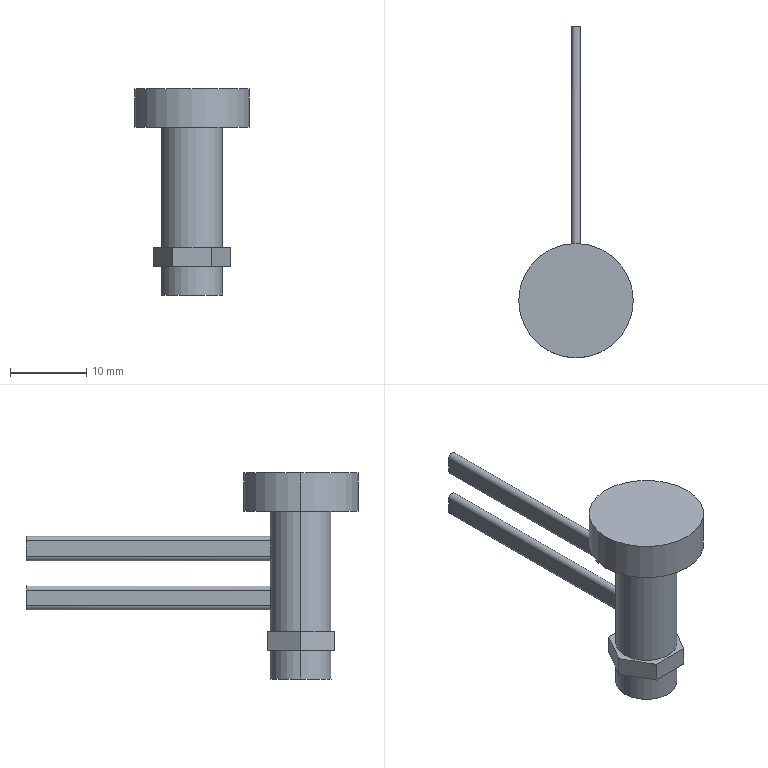Part | SolidWorks | features BaseBody 1 | 1 solid | 29 faces | box 15 x 43.5 x 27 mm | volume 2257 mm3 | plane 17 | cylinder 12 | commonest cylinder face diameters 1.197 x6 8 x4 15 x2
STEP:
#1=CARTESIAN_POINT('',(0.,36.,-12.942));
#2=VERTEX_POINT('',#1);
#3=CARTESIAN_POINT('',(-0.5985,36.,-12.344));
#4=VERTEX_POINT('',#3);
#5=CARTESIAN_POINT('',(0.,36.,-12.344));
#6=DIRECTION('',(0.,1.,0.));
#7=DIRECTION('',(0.,0.,1.));
#8=AXIS2_PLACEMENT_3D('',#5,#6,#7);
#9=CIRCLE('',#8,0.5985);
#10=EDGE_CURVE('',#2,#4,#9,.T.);
#11=ORIENTED_EDGE('',*,*,#10,.F.);
#12=CARTESIAN_POINT('',(0.,4.,-12.942));
#13=VERTEX_POINT('',#12);
#14=CARTESIAN_POINT('',(0.,36.,-12.942));
#15=DIRECTION('',(0.,-1.,0.));
#16=VECTOR('',#15,1000.);
#17=LINE('',#14,#16);
#18=EDGE_CURVE('',#2,#13,#17,.T.);
#19=ORIENTED_EDGE('',*,*,#18,.T.);
#20=CARTESIAN_POINT('',(-0.5985,3.955,-12.344));
#21=VERTEX_POINT('',#20);
#22=CARTESIAN_POINT('',(0.,4.,-12.942));
#23=CARTESIAN_POINT('',(-0.1585,4.,-12.942));
#24=CARTESIAN_POINT('',(-0.3131,3.989,-12.877));
#25=CARTESIAN_POINT('',(-0.5336,3.966,-12.657));
#26=CARTESIAN_POINT('',(-0.5985,3.955,-12.5));
#27=CARTESIAN_POINT('',(-0.5985,3.955,-12.344));
#28=B_SPLINE_CURVE_WITH_KNOTS('',3,(#22,#23,#24,#25,#26,#27),.UNSPECIFIED.,.F.,.F.,(4,2,4),(0.,0.0004686,0.0009371),.UNSPECIFIED.);
#29=EDGE_CURVE('',#13,#21,#28,.T.);
#30=ORIENTED_EDGE('',*,*,#29,.T.);
#31=CARTESIAN_POINT('',(-0.5985,36.,-12.344));
#32=DIRECTION('',(0.,-1.,0.));
#33=VECTOR('',#32,1000.);
#34=LINE('',#31,#33);
#35=EDGE_CURVE('',#4,#21,#34,.T.);
#36=ORIENTED_EDGE('',*,*,#35,.F.);
#37=EDGE_LOOP('',(#11,#19,#30,#36));
#38=FACE_OUTER_BOUND('',#37,.T.);
#39=CARTESIAN_POINT('',(0.,36.,-12.344));
#40=DIRECTION('',(0.,-1.,0.));
#41=DIRECTION('',(0.,0.,-1.));
#42=AXIS2_PLACEMENT_3D('',#39,#40,#41);
#43=CYLINDRICAL_SURFACE('',#42,0.5985);
#44=ADVANCED_FACE('',(#38),#43,.T.);
#45=CARTESIAN_POINT('',(0.,36.,-6.501));
#46=VERTEX_POINT('',#45);
#47=CARTESIAN_POINT('',(-0.5985,36.,-5.903));
#48=VERTEX_POINT('',#47);
#49=CARTESIAN_POINT('',(0.,36.,-5.903));
#50=DIRECTION('',(0.,1.,0.));
#51=DIRECTION('',(0.,0.,1.));
#52=AXIS2_PLACEMENT_3D('',#49,#50,#51);
#53=CIRCLE('',#52,0.5985);
#54=EDGE_CURVE('',#46,#48,#53,.T.);
#55=ORIENTED_EDGE('',*,*,#54,.F.);
#56=CARTESIAN_POINT('',(0.,4.,-6.501));
#57=VERTEX_POINT('',#56);
#58=CARTESIAN_POINT('',(0.,36.,-6.501));
#59=DIRECTION('',(0.,-1.,0.));
#60=VECTOR('',#59,1000.);
#61=LINE('',#58,#60);
#62=EDGE_CURVE('',#46,#57,#61,.T.);
#63=ORIENTED_EDGE('',*,*,#62,.T.);
#64=CARTESIAN_POINT('',(-0.5985,3.955,-5.903));
#65=VERTEX_POINT('',#64);
#66=CARTESIAN_POINT('',(0.,4.,-6.501));
#67=CARTESIAN_POINT('',(-0.1585,4.,-6.501));
#68=CARTESIAN_POINT('',(-0.3131,3.989,-6.436));
#69=CARTESIAN_POINT('',(-0.5336,3.966,-6.216));
#70=CARTESIAN_POINT('',(-0.5985,3.955,-6.059));
#71=CARTESIAN_POINT('',(-0.5985,3.955,-5.903));
#72=B_SPLINE_CURVE_WITH_KNOTS('',3,(#66,#67,#68,#69,#70,#71),.UNSPECIFIED.,.F.,.F.,(4,2,4),(0.,0.0004686,0.0009371),.UNSPECIFIED.);
#73=EDGE_CURVE('',#57,#65,#72,.T.);
#74=ORIENTED_EDGE('',*,*,#73,.T.);
#75=CARTESIAN_POINT('',(-0.5985,36.,-5.903));
#76=DIRECTION('',(0.,-1.,0.));
#77=VECTOR('',#76,1000.);
#78=LINE('',#75,#77);
#79=EDGE_CURVE('',#48,#65,#78,.T.);
#80=ORIENTED_EDGE('',*,*,#79,.F.);
#81=EDGE_LOOP('',(#55,#63,#74,#80));
#82=FACE_OUTER_BOUND('',#81,.T.);
#83=CARTESIAN_POINT('',(0.,36.,-5.903));
#84=DIRECTION('',(0.,-1.,0.));
#85=DIRECTION('',(0.,0.,-1.));
#86=AXIS2_PLACEMENT_3D('',#83,#84,#85);
#87=CYLINDRICAL_SURFACE('',#86,0.5985);
#88=ADVANCED_FACE('',(#82),#87,.T.);
#89=CARTESIAN_POINT('',(-4.,0.,-22.));
#90=VERTEX_POINT('',#89);
#91=CARTESIAN_POINT('',(4.,0.,-22.));
#92=VERTEX_POINT('',#91);
#93=CARTESIAN_POINT('',(0.,0.,-22.));
#94=DIRECTION('',(0.,0.,-1.));
#95=DIRECTION('',(-1.,0.,0.));
#96=AXIS2_PLACEMENT_3D('',#93,#94,#95);
#97=CIRCLE('',#96,4.);
#98=EDGE_CURVE('',#90,#92,#97,.T.);
#99=ORIENTED_EDGE('',*,*,#98,.F.);
#100=CARTESIAN_POINT('',(-4.,0.,-18.25));
#101=VERTEX_POINT('',#100);
#102=CARTESIAN_POINT('',(-4.,0.,-22.));
#103=DIRECTION('',(0.,0.,1.));
#104=VECTOR('',#103,1000.);
#105=LINE('',#102,#104);
#106=EDGE_CURVE('',#90,#101,#105,.T.);
#107=ORIENTED_EDGE('',*,*,#106,.T.);
#108=CARTESIAN_POINT('',(4.,0.,-18.25));
#109=VERTEX_POINT('',#108);
#110=CARTESIAN_POINT('',(0.,0.,-18.25));
#111=DIRECTION('',(0.,0.,-1.));
#112=DIRECTION('',(-1.,0.,0.));
#113=AXIS2_PLACEMENT_3D('',#110,#111,#112);
#114=CIRCLE('',#113,4.);
#115=EDGE_CURVE('',#101,#109,#114,.T.);
#116=ORIENTED_EDGE('',*,*,#115,.T.);
#117=CARTESIAN_POINT('',(4.,0.,-22.));
#118=DIRECTION('',(0.,0.,1.));
#119=VECTOR('',#118,1000.);
#120=LINE('',#117,#119);
#121=EDGE_CURVE('',#92,#109,#120,.T.);
#122=ORIENTED_EDGE('',*,*,#121,.F.);
#123=EDGE_LOOP('',(#99,#107,#116,#122));
#124=FACE_OUTER_BOUND('',#123,.T.);
#125=CARTESIAN_POINT('',(0.,0.,-22.));
#126=DIRECTION('',(0.,0.,1.));
#127=DIRECTION('',(1.,0.,0.));
#128=AXIS2_PLACEMENT_3D('',#125,#126,#127);
#129=CYLINDRICAL_SURFACE('',#128,4.);
#130=ADVANCED_FACE('',(#124),#129,.T.);
#131=CARTESIAN_POINT('',(7.5,0.,5.));
#132=VERTEX_POINT('',#131);
#133=CARTESIAN_POINT('',(-7.5,0.,5.));
#134=VERTEX_POINT('',#133);
#135=CARTESIAN_POINT('',(0.,0.,5.));
#136=DIRECTION('',(0.,0.,1.));
#137=DIRECTION('',(1.,0.,0.));
#138=AXIS2_PLACEMENT_3D('',#135,#136,#137);
#139=CIRCLE('',#138,7.5);
#140=EDGE_CURVE('',#132,#134,#139,.T.);
#141=ORIENTED_EDGE('',*,*,#140,.F.);
#142=CARTESIAN_POINT('',(7.5,0.,0.));
#143=VERTEX_POINT('',#142);
#144=CARTESIAN_POINT('',(7.5,0.,5.));
#145=DIRECTION('',(0.,0.,-1.));
#146=VECTOR('',#145,1000.);
#147=LINE('',#144,#146);
#148=EDGE_CURVE('',#132,#143,#147,.T.);
#149=ORIENTED_EDGE('',*,*,#148,.T.);
#150=CARTESIAN_POINT('',(-7.5,0.,0.));
#151=VERTEX_POINT('',#150);
#152=CARTESIAN_POINT('',(0.,0.,0.));
#153=DIRECTION('',(0.,0.,1.));
#154=DIRECTION('',(1.,0.,0.));
#155=AXIS2_PLACEMENT_3D('',#152,#153,#154);
#156=CIRCLE('',#155,7.5);
#157=EDGE_CURVE('',#143,#151,#156,.T.);
#158=ORIENTED_EDGE('',*,*,#157,.T.);
#159=CARTESIAN_POINT('',(-7.5,0.,5.));
#160=DIRECTION('',(0.,0.,-1.));
#161=VECTOR('',#160,1000.);
#162=LINE('',#159,#161);
#163=EDGE_CURVE('',#134,#151,#162,.T.);
#164=ORIENTED_EDGE('',*,*,#163,.F.);
#165=EDGE_LOOP('',(#141,#149,#158,#164));
#166=FACE_OUTER_BOUND('',#165,.T.);
#167=CARTESIAN_POINT('',(0.,0.,5.));
#168=DIRECTION('',(0.,0.,-1.));
#169=DIRECTION('',(-1.,0.,0.));
#170=AXIS2_PLACEMENT_3D('',#167,#168,#169);
#171=CYLINDRICAL_SURFACE('',#170,7.5);
#172=ADVANCED_FACE('',(#166),#171,.T.);
#173=CARTESIAN_POINT('',(-0.5985,3.955,-3.903));
#174=VERTEX_POINT('',#173);
#175=CARTESIAN_POINT('',(0.5985,3.955,-3.903));
#176=VERTEX_POINT('',#175);
#177=CARTESIAN_POINT('',(-0.5985,3.955,-3.903));
#178=CARTESIAN_POINT('',(-0.5985,3.955,-3.746));
#179=CARTESIAN_POINT('',(-0.5347,3.966,-3.591));
#180=CARTESIAN_POINT('',(-0.3115,3.989,-3.368));
#181=CARTESIAN_POINT('',(-0.1562,4.,-3.304));
#182=CARTESIAN_POINT('',(0.1565,4.,-3.304));
#183=CARTESIAN_POINT('',(0.3128,3.989,-3.369));
#184=CARTESIAN_POINT('',(0.5335,3.966,-3.59));
#185=CARTESIAN_POINT('',(0.5985,3.955,-3.745));
#186=CARTESIAN_POINT('',(0.5985,3.955,-3.903));
#187=B_SPLINE_CURVE_WITH_KNOTS('',3,(#177,#178,#179,#180,#181,#182,#183,#184,#185,#186),.UNSPECIFIED.,.F.,.F.,(4,2,2,2,4),(0.0009371,0.001406,0.001874,0.002342,0.002811),.UNSPECIFIED.);
#188=EDGE_CURVE('',#174,#176,#187,.T.);
#189=ORIENTED_EDGE('',*,*,#188,.F.);
#190=CARTESIAN_POINT('',(-0.5985,3.955,-22.));
#191=DIRECTION('',(0.,0.,1.));
#192=VECTOR('',#191,1000.);
#193=LINE('',#190,#192);
#194=EDGE_CURVE('',#65,#174,#193,.T.);
#195=ORIENTED_EDGE('',*,*,#194,.F.);
#196=ORIENTED_EDGE('',*,*,#73,.F.);
#197=CARTESIAN_POINT('',(0.5985,3.955,-5.903));
#198=VERTEX_POINT('',#197);
#199=CARTESIAN_POINT('',(0.5985,3.955,-5.903));
#200=CARTESIAN_POINT('',(0.5985,3.955,-6.061));
#201=CARTESIAN_POINT('',(0.5335,3.966,-6.216));
#202=CARTESIAN_POINT('',(0.3132,3.989,-6.436));
#203=CARTESIAN_POINT('',(0.1583,4.,-6.501));
#204=CARTESIAN_POINT('',(0.,4.,-6.501));
#205=B_SPLINE_CURVE_WITH_KNOTS('',3,(#199,#200,#201,#202,#203,#204),.UNSPECIFIED.,.F.,.F.,(4,2,4),(0.002811,0.003279,0.003747),.UNSPECIFIED.);
#206=EDGE_CURVE('',#198,#57,#205,.T.);
#207=ORIENTED_EDGE('',*,*,#206,.F.);
#208=CARTESIAN_POINT('',(0.5985,3.955,-22.));
#209=DIRECTION('',(0.,0.,-1.));
#210=VECTOR('',#209,1000.);
#211=LINE('',#208,#210);
#212=EDGE_CURVE('',#176,#198,#211,.T.);
#213=ORIENTED_EDGE('',*,*,#212,.F.);
#214=EDGE_LOOP('',(#189,#195,#196,#207,#213));
#215=FACE_BOUND('',#214,.T.);
#216=CARTESIAN_POINT('',(-0.5985,3.955,-10.344));
#217=VERTEX_POINT('',#216);
#218=CARTESIAN_POINT('',(0.5985,3.955,-10.344));
#219=VERTEX_POINT('',#218);
#220=CARTESIAN_POINT('',(-0.5985,3.955,-10.344));
#221=CARTESIAN_POINT('',(-0.5985,3.955,-10.187));
#222=CARTESIAN_POINT('',(-0.5347,3.966,-10.032));
#223=CARTESIAN_POINT('',(-0.3115,3.989,-9.809));
#224=CARTESIAN_POINT('',(-0.1562,4.,-9.745));
#225=CARTESIAN_POINT('',(0.1565,4.,-9.745));
#226=CARTESIAN_POINT('',(0.3128,3.989,-9.81));
#227=CARTESIAN_POINT('',(0.5335,3.966,-10.031));
#228=CARTESIAN_POINT('',(0.5985,3.955,-10.186));
#229=CARTESIAN_POINT('',(0.5985,3.955,-10.344));
#230=B_SPLINE_CURVE_WITH_KNOTS('',3,(#220,#221,#222,#223,#224,#225,#226,#227,#228,#229),.UNSPECIFIED.,.F.,.F.,(4,2,2,2,4),(0.0009371,0.001406,0.001874,0.002342,0.002811),.UNSPECIFIED.);
#231=EDGE_CURVE('',#217,#219,#230,.T.);
#232=ORIENTED_EDGE('',*,*,#231,.F.);
#233=CARTESIAN_POINT('',(-0.5985,3.955,-22.));
#234=DIRECTION('',(0.,0.,1.));
#235=VECTOR('',#234,1000.);
#236=LINE('',#233,#235);
#237=EDGE_CURVE('',#21,#217,#236,.T.);
#238=ORIENTED_EDGE('',*,*,#237,.F.);
#239=ORIENTED_EDGE('',*,*,#29,.F.);
#240=CARTESIAN_POINT('',(0.5985,3.955,-12.344));
#241=VERTEX_POINT('',#240);
#242=CARTESIAN_POINT('',(0.5985,3.955,-12.344));
#243=CARTESIAN_POINT('',(0.5985,3.955,-12.502));
#244=CARTESIAN_POINT('',(0.5335,3.966,-12.657));
#245=CARTESIAN_POINT('',(0.3132,3.989,-12.877));
#246=CARTESIAN_POINT('',(0.1583,4.,-12.942));
#247=CARTESIAN_POINT('',(0.,4.,-12.942));
#248=B_SPLINE_CURVE_WITH_KNOTS('',3,(#242,#243,#244,#245,#246,#247),.UNSPECIFIED.,.F.,.F.,(4,2,4),(0.002811,0.003279,0.003747),.UNSPECIFIED.);
#249=EDGE_CURVE('',#241,#13,#248,.T.);
#250=ORIENTED_EDGE('',*,*,#249,.F.);
#251=CARTESIAN_POINT('',(0.5985,3.955,-22.));
#252=DIRECTION('',(0.,0.,-1.));
#253=VECTOR('',#252,1000.);
#254=LINE('',#251,#253);
#255=EDGE_CURVE('',#219,#241,#254,.T.);
#256=ORIENTED_EDGE('',*,*,#255,.F.);
#257=EDGE_LOOP('',(#232,#238,#239,#250,#256));
#258=FACE_BOUND('',#257,.T.);
#259=CARTESIAN_POINT('',(-4.,0.,-15.75));
#260=VERTEX_POINT('',#259);
#261=CARTESIAN_POINT('',(4.,0.,-15.75));
#262=VERTEX_POINT('',#261);
#263=CARTESIAN_POINT('',(0.,0.,-15.75));
#264=DIRECTION('',(0.,0.,-1.));
#265=DIRECTION('',(-1.,0.,0.));
#266=AXIS2_PLACEMENT_3D('',#263,#264,#265);
#267=CIRCLE('',#266,4.);
#268=EDGE_CURVE('',#260,#262,#267,.T.);
#269=ORIENTED_EDGE('',*,*,#268,.F.);
#270=CARTESIAN_POINT('',(-4.,0.,0.));
#271=VERTEX_POINT('',#270);
#272=CARTESIAN_POINT('',(-4.,0.,-22.));
#273=DIRECTION('',(0.,0.,1.));
#274=VECTOR('',#273,1000.);
#275=LINE('',#272,#274);
#276=EDGE_CURVE('',#260,#271,#275,.T.);
#277=ORIENTED_EDGE('',*,*,#276,.T.);
#278=CARTESIAN_POINT('',(4.,0.,0.));
#279=VERTEX_POINT('',#278);
#280=CARTESIAN_POINT('',(0.,0.,0.));
#281=DIRECTION('',(0.,0.,-1.));
#282=DIRECTION('',(-1.,0.,0.));
#283=AXIS2_PLACEMENT_3D('',#280,#281,#282);
#284=CIRCLE('',#283,4.);
#285=EDGE_CURVE('',#271,#279,#284,.T.);
#286=ORIENTED_EDGE('',*,*,#285,.T.);
#287=CARTESIAN_POINT('',(4.,0.,-22.));
#288=DIRECTION('',(0.,0.,1.));
#289=VECTOR('',#288,1000.);
#290=LINE('',#287,#289);
#291=EDGE_CURVE('',#262,#279,#290,.T.);
#292=ORIENTED_EDGE('',*,*,#291,.F.);
#293=EDGE_LOOP('',(#269,#277,#286,#292));
#294=FACE_OUTER_BOUND('',#293,.T.);
#295=CARTESIAN_POINT('',(0.,0.,-22.));
#296=DIRECTION('',(0.,0.,1.));
#297=DIRECTION('',(1.,0.,0.));
#298=AXIS2_PLACEMENT_3D('',#295,#296,#297);
#299=CYLINDRICAL_SURFACE('',#298,4.);
#300=ADVANCED_FACE('',(#215,#258,#294),#299,.T.);
#301=ORIENTED_EDGE('',*,*,#276,.F.);
#302=CARTESIAN_POINT('',(0.,0.,-15.75));
#303=DIRECTION('',(0.,0.,-1.));
#304=DIRECTION('',(-1.,0.,0.));
#305=AXIS2_PLACEMENT_3D('',#302,#303,#304);
#306=CIRCLE('',#305,4.);
#307=EDGE_CURVE('',#262,#260,#306,.T.);
#308=ORIENTED_EDGE('',*,*,#307,.F.);
#309=ORIENTED_EDGE('',*,*,#291,.T.);
#310=CARTESIAN_POINT('',(0.,0.,0.));
#311=DIRECTION('',(0.,0.,-1.));
#312=DIRECTION('',(-1.,0.,0.));
#313=AXIS2_PLACEMENT_3D('',#310,#311,#312);
#314=CIRCLE('',#313,4.);
#315=EDGE_CURVE('',#279,#271,#314,.T.);
#316=ORIENTED_EDGE('',*,*,#315,.T.);
#317=EDGE_LOOP('',(#301,#308,#309,#316));
#318=FACE_OUTER_BOUND('',#317,.T.);
#319=CARTESIAN_POINT('',(0.,0.,-22.));
#320=DIRECTION('',(0.,0.,1.));
#321=DIRECTION('',(1.,0.,0.));
#322=AXIS2_PLACEMENT_3D('',#319,#320,#321);
#323=CYLINDRICAL_SURFACE('',#322,4.);
#324=ADVANCED_FACE('',(#318),#323,.T.);
#325=ORIENTED_EDGE('',*,*,#148,.F.);
#326=CARTESIAN_POINT('',(0.,0.,5.));
#327=DIRECTION('',(0.,0.,1.));
#328=DIRECTION('',(1.,0.,0.));
#329=AXIS2_PLACEMENT_3D('',#326,#327,#328);
#330=CIRCLE('',#329,7.5);
#331=EDGE_CURVE('',#134,#132,#330,.T.);
#332=ORIENTED_EDGE('',*,*,#331,.F.);
#333=ORIENTED_EDGE('',*,*,#163,.T.);
#334=CARTESIAN_POINT('',(0.,0.,0.));
#335=DIRECTION('',(0.,0.,1.));
#336=DIRECTION('',(1.,0.,0.));
#337=AXIS2_PLACEMENT_3D('',#334,#335,#336);
#338=CIRCLE('',#337,7.5);
#339=EDGE_CURVE('',#151,#143,#338,.T.);
#340=ORIENTED_EDGE('',*,*,#339,.T.);
#341=EDGE_LOOP('',(#325,#332,#333,#340));
#342=FACE_OUTER_BOUND('',#341,.T.);
#343=CARTESIAN_POINT('',(0.,0.,5.));
#344=DIRECTION('',(0.,0.,-1.));
#345=DIRECTION('',(-1.,0.,0.));
#346=AXIS2_PLACEMENT_3D('',#343,#344,#345);
#347=CYLINDRICAL_SURFACE('',#346,7.5);
#348=ADVANCED_FACE('',(#342),#347,.T.);
#349=ORIENTED_EDGE('',*,*,#331,.T.);
#350=ORIENTED_EDGE('',*,*,#140,.T.);
#351=EDGE_LOOP('',(#349,#350));
#352=FACE_OUTER_BOUND('',#351,.T.);
#353=CARTESIAN_POINT('',(0.,0.,5.));
#354=DIRECTION('',(0.,0.,1.));
#355=DIRECTION('',(1.,0.,0.));
#356=AXIS2_PLACEMENT_3D('',#353,#354,#355);
#357=PLANE('',#356);
#358=ADVANCED_FACE('',(#352),#357,.T.);
#359=ORIENTED_EDGE('',*,*,#315,.F.);
#360=ORIENTED_EDGE('',*,*,#285,.F.);
#361=EDGE_LOOP('',(#359,#360));
#362=FACE_BOUND('',#361,.T.);
#363=ORIENTED_EDGE('',*,*,#339,.F.);
#364=ORIENTED_EDGE('',*,*,#157,.F.);
#365=EDGE_LOOP('',(#363,#364));
#366=FACE_OUTER_BOUND('',#365,.T.);
#367=CARTESIAN_POINT('',(0.,0.,0.));
#368=DIRECTION('',(0.,0.,1.));
#369=DIRECTION('',(1.,0.,0.));
#370=AXIS2_PLACEMENT_3D('',#367,#368,#369);
#371=PLANE('',#370);
#372=ADVANCED_FACE('',(#362,#366),#371,.F.);
#373=CARTESIAN_POINT('',(-2.541,-4.402,-15.75));
#374=VERTEX_POINT('',#373);
#375=CARTESIAN_POINT('',(-5.083,0.,-15.75));
#376=VERTEX_POINT('',#375);
#377=CARTESIAN_POINT('',(-2.541,-4.402,-15.75));
#378=DIRECTION('',(-0.5,0.866,0.));
#379=VECTOR('',#378,1000.);
#380=LINE('',#377,#379);
#381=EDGE_CURVE('',#374,#376,#380,.T.);
#382=ORIENTED_EDGE('',*,*,#381,.T.);
#383=CARTESIAN_POINT('',(-5.083,0.,-18.25));
#384=VERTEX_POINT('',#383);
#385=CARTESIAN_POINT('',(-5.083,0.,-18.25));
#386=DIRECTION('',(0.,0.,1.));
#387=VECTOR('',#386,1000.);
#388=LINE('',#385,#387);
#389=EDGE_CURVE('',#384,#376,#388,.T.);
#390=ORIENTED_EDGE('',*,*,#389,.F.);
#391=CARTESIAN_POINT('',(-2.541,-4.402,-18.25));
#392=VERTEX_POINT('',#391);
#393=CARTESIAN_POINT('',(-2.541,-4.402,-18.25));
#394=DIRECTION('',(-0.5,0.866,0.));
#395=VECTOR('',#394,1000.);
#396=LINE('',#393,#395);
#397=EDGE_CURVE('',#392,#384,#396,.T.);
#398=ORIENTED_EDGE('',*,*,#397,.F.);
#399=CARTESIAN_POINT('',(-2.541,-4.402,-18.25));
#400=DIRECTION('',(0.,0.,1.));
#401=VECTOR('',#400,1000.);
#402=LINE('',#399,#401);
#403=EDGE_CURVE('',#392,#374,#402,.T.);
#404=ORIENTED_EDGE('',*,*,#403,.T.);
#405=EDGE_LOOP('',(#382,#390,#398,#404));
#406=FACE_OUTER_BOUND('',#405,.T.);
#407=CARTESIAN_POINT('',(-2.541,-4.402,-18.25));
#408=DIRECTION('',(0.866,0.5,0.));
#409=DIRECTION('',(-0.5,0.866,0.));
#410=AXIS2_PLACEMENT_3D('',#407,#408,#409);
#411=PLANE('',#410);
#412=ADVANCED_FACE('',(#406),#411,.F.);
#413=CARTESIAN_POINT('',(-2.541,4.402,-15.75));
#414=VERTEX_POINT('',#413);
#415=CARTESIAN_POINT('',(-5.083,0.,-15.75));
#416=DIRECTION('',(0.5,0.866,0.));
#417=VECTOR('',#416,1000.);
#418=LINE('',#415,#417);
#419=EDGE_CURVE('',#376,#414,#418,.T.);
#420=ORIENTED_EDGE('',*,*,#419,.T.);
#421=CARTESIAN_POINT('',(-2.541,4.402,-18.25));
#422=VERTEX_POINT('',#421);
#423=CARTESIAN_POINT('',(-2.541,4.402,-18.25));
#424=DIRECTION('',(0.,0.,1.));
#425=VECTOR('',#424,1000.);
#426=LINE('',#423,#425);
#427=EDGE_CURVE('',#422,#414,#426,.T.);
#428=ORIENTED_EDGE('',*,*,#427,.F.);
#429=CARTESIAN_POINT('',(-5.083,0.,-18.25));
#430=DIRECTION('',(0.5,0.866,0.));
#431=VECTOR('',#430,1000.);
#432=LINE('',#429,#431);
#433=EDGE_CURVE('',#384,#422,#432,.T.);
#434=ORIENTED_EDGE('',*,*,#433,.F.);
#435=ORIENTED_EDGE('',*,*,#389,.T.);
#436=EDGE_LOOP('',(#420,#428,#434,#435));
#437=FACE_OUTER_BOUND('',#436,.T.);
#438=CARTESIAN_POINT('',(-5.083,0.,-18.25));
#439=DIRECTION('',(0.866,-0.5,0.));
#440=DIRECTION('',(0.5,0.866,0.));
#441=AXIS2_PLACEMENT_3D('',#438,#439,#440);
#442=PLANE('',#441);
#443=ADVANCED_FACE('',(#437),#442,.F.);
#444=CARTESIAN_POINT('',(2.541,4.402,-15.75));
#445=VERTEX_POINT('',#444);
#446=CARTESIAN_POINT('',(-2.541,4.402,-15.75));
#447=DIRECTION('',(1.,0.,0.));
#448=VECTOR('',#447,1000.);
#449=LINE('',#446,#448);
#450=EDGE_CURVE('',#414,#445,#449,.T.);
#451=ORIENTED_EDGE('',*,*,#450,.T.);
#452=CARTESIAN_POINT('',(2.541,4.402,-18.25));
#453=VERTEX_POINT('',#452);
#454=CARTESIAN_POINT('',(2.541,4.402,-18.25));
#455=DIRECTION('',(0.,0.,1.));
#456=VECTOR('',#455,1000.);
#457=LINE('',#454,#456);
#458=EDGE_CURVE('',#453,#445,#457,.T.);
#459=ORIENTED_EDGE('',*,*,#458,.F.);
#460=CARTESIAN_POINT('',(-2.541,4.402,-18.25));
#461=DIRECTION('',(1.,0.,0.));
#462=VECTOR('',#461,1000.);
#463=LINE('',#460,#462);
#464=EDGE_CURVE('',#422,#453,#463,.T.);
#465=ORIENTED_EDGE('',*,*,#464,.F.);
#466=ORIENTED_EDGE('',*,*,#427,.T.);
#467=EDGE_LOOP('',(#451,#459,#465,#466));
#468=FACE_OUTER_BOUND('',#467,.T.);
#469=CARTESIAN_POINT('',(-2.541,4.402,-18.25));
#470=DIRECTION('',(0.,-1.,0.));
#471=DIRECTION('',(1.,0.,0.));
#472=AXIS2_PLACEMENT_3D('',#469,#470,#471);
#473=PLANE('',#472);
#474=ADVANCED_FACE('',(#468),#473,.F.);
#475=CARTESIAN_POINT('',(5.083,0.,-15.75));
#476=VERTEX_POINT('',#475);
#477=CARTESIAN_POINT('',(2.541,4.402,-15.75));
#478=DIRECTION('',(0.5,-0.866,0.));
#479=VECTOR('',#478,1000.);
#480=LINE('',#477,#479);
#481=EDGE_CURVE('',#445,#476,#480,.T.);
#482=ORIENTED_EDGE('',*,*,#481,.T.);
#483=CARTESIAN_POINT('',(5.083,0.,-18.25));
#484=VERTEX_POINT('',#483);
#485=CARTESIAN_POINT('',(5.083,0.,-18.25));
#486=DIRECTION('',(0.,0.,1.));
#487=VECTOR('',#486,1000.);
#488=LINE('',#485,#487);
#489=EDGE_CURVE('',#484,#476,#488,.T.);
#490=ORIENTED_EDGE('',*,*,#489,.F.);
#491=CARTESIAN_POINT('',(2.541,4.402,-18.25));
#492=DIRECTION('',(0.5,-0.866,0.));
#493=VECTOR('',#492,1000.);
#494=LINE('',#491,#493);
#495=EDGE_CURVE('',#453,#484,#494,.T.);
#496=ORIENTED_EDGE('',*,*,#495,.F.);
#497=ORIENTED_EDGE('',*,*,#458,.T.);
#498=EDGE_LOOP('',(#482,#490,#496,#497));
#499=FACE_OUTER_BOUND('',#498,.T.);
#500=CARTESIAN_POINT('',(2.541,4.402,-18.25));
#501=DIRECTION('',(-0.866,-0.5,0.));
#502=DIRECTION('',(0.5,-0.866,0.));
#503=AXIS2_PLACEMENT_3D('',#500,#501,#502);
#504=PLANE('',#503);
#505=ADVANCED_FACE('',(#499),#504,.F.);
#506=CARTESIAN_POINT('',(2.541,-4.402,-15.75));
#507=VERTEX_POINT('',#506);
#508=CARTESIAN_POINT('',(5.083,0.,-15.75));
#509=DIRECTION('',(-0.5,-0.866,0.));
#510=VECTOR('',#509,1000.);
#511=LINE('',#508,#510);
#512=EDGE_CURVE('',#476,#507,#511,.T.);
#513=ORIENTED_EDGE('',*,*,#512,.T.);
#514=CARTESIAN_POINT('',(2.541,-4.402,-18.25));
#515=VERTEX_POINT('',#514);
#516=CARTESIAN_POINT('',(2.541,-4.402,-18.25));
#517=DIRECTION('',(0.,0.,1.));
#518=VECTOR('',#517,1000.);
#519=LINE('',#516,#518);
#520=EDGE_CURVE('',#515,#507,#519,.T.);
#521=ORIENTED_EDGE('',*,*,#520,.F.);
#522=CARTESIAN_POINT('',(5.083,0.,-18.25));
#523=DIRECTION('',(-0.5,-0.866,0.));
#524=VECTOR('',#523,1000.);
#525=LINE('',#522,#524);
#526=EDGE_CURVE('',#484,#515,#525,.T.);
#527=ORIENTED_EDGE('',*,*,#526,.F.);
#528=ORIENTED_EDGE('',*,*,#489,.T.);
#529=EDGE_LOOP('',(#513,#521,#527,#528));
#530=FACE_OUTER_BOUND('',#529,.T.);
#531=CARTESIAN_POINT('',(5.083,0.,-18.25));
#532=DIRECTION('',(-0.866,0.5,0.));
#533=DIRECTION('',(-0.5,-0.866,0.));
#534=AXIS2_PLACEMENT_3D('',#531,#532,#533);
#535=PLANE('',#534);
#536=ADVANCED_FACE('',(#530),#535,.F.);
#537=CARTESIAN_POINT('',(2.541,-4.402,-15.75));
#538=DIRECTION('',(-1.,0.,0.));
#539=VECTOR('',#538,1000.);
#540=LINE('',#537,#539);
#541=EDGE_CURVE('',#507,#374,#540,.T.);
#542=ORIENTED_EDGE('',*,*,#541,.T.);
#543=ORIENTED_EDGE('',*,*,#403,.F.);
#544=CARTESIAN_POINT('',(2.541,-4.402,-18.25));
#545=DIRECTION('',(-1.,0.,0.));
#546=VECTOR('',#545,1000.);
#547=LINE('',#544,#546);
#548=EDGE_CURVE('',#515,#392,#547,.T.);
#549=ORIENTED_EDGE('',*,*,#548,.F.);
#550=ORIENTED_EDGE('',*,*,#520,.T.);
#551=EDGE_LOOP('',(#542,#543,#549,#550));
#552=FACE_OUTER_BOUND('',#551,.T.);
#553=CARTESIAN_POINT('',(2.541,-4.402,-18.25));
#554=DIRECTION('',(0.,1.,0.));
#555=DIRECTION('',(-1.,0.,0.));
#556=AXIS2_PLACEMENT_3D('',#553,#554,#555);
#557=PLANE('',#556);
#558=ADVANCED_FACE('',(#552),#557,.F.);
#559=CARTESIAN_POINT('',(0.,0.,-18.25));
#560=DIRECTION('',(0.,0.,-1.));
#561=DIRECTION('',(-1.,0.,0.));
#562=AXIS2_PLACEMENT_3D('',#559,#560,#561);
#563=CIRCLE('',#562,4.);
#564=EDGE_CURVE('',#109,#101,#563,.T.);
#565=ORIENTED_EDGE('',*,*,#564,.F.);
#566=ORIENTED_EDGE('',*,*,#115,.F.);
#567=EDGE_LOOP('',(#565,#566));
#568=FACE_BOUND('',#567,.T.);
#569=ORIENTED_EDGE('',*,*,#397,.T.);
#570=ORIENTED_EDGE('',*,*,#433,.T.);
#571=ORIENTED_EDGE('',*,*,#464,.T.);
#572=ORIENTED_EDGE('',*,*,#495,.T.);
#573=ORIENTED_EDGE('',*,*,#526,.T.);
#574=ORIENTED_EDGE('',*,*,#548,.T.);
#575=EDGE_LOOP('',(#569,#570,#571,#572,#573,#574));
#576=FACE_OUTER_BOUND('',#575,.T.);
#577=CARTESIAN_POINT('',(0.,0.,-18.25));
#578=DIRECTION('',(0.,0.,-1.));
#579=DIRECTION('',(-1.,0.,0.));
#580=AXIS2_PLACEMENT_3D('',#577,#578,#579);
#581=PLANE('',#580);
#582=ADVANCED_FACE('',(#568,#576),#581,.T.);
#583=ORIENTED_EDGE('',*,*,#307,.T.);
#584=ORIENTED_EDGE('',*,*,#268,.T.);
#585=EDGE_LOOP('',(#583,#584));
#586=FACE_BOUND('',#585,.T.);
#587=ORIENTED_EDGE('',*,*,#381,.F.);
#588=ORIENTED_EDGE('',*,*,#541,.F.);
#589=ORIENTED_EDGE('',*,*,#512,.F.);
#590=ORIENTED_EDGE('',*,*,#481,.F.);
#591=ORIENTED_EDGE('',*,*,#450,.F.);
#592=ORIENTED_EDGE('',*,*,#419,.F.);
#593=EDGE_LOOP('',(#587,#588,#589,#590,#591,#592));
#594=FACE_OUTER_BOUND('',#593,.T.);
#595=CARTESIAN_POINT('',(0.,0.,-15.75));
#596=DIRECTION('',(0.,0.,-1.));
#597=DIRECTION('',(-1.,0.,0.));
#598=AXIS2_PLACEMENT_3D('',#595,#596,#597);
#599=PLANE('',#598);
#600=ADVANCED_FACE('',(#586,#594),#599,.F.);
#601=CARTESIAN_POINT('',(0.,0.,-22.));
#602=DIRECTION('',(0.,0.,-1.));
#603=DIRECTION('',(-1.,0.,0.));
#604=AXIS2_PLACEMENT_3D('',#601,#602,#603);
#605=CIRCLE('',#604,4.);
#606=EDGE_CURVE('',#92,#90,#605,.T.);
#607=ORIENTED_EDGE('',*,*,#606,.T.);
#608=ORIENTED_EDGE('',*,*,#98,.T.);
#609=EDGE_LOOP('',(#607,#608));
#610=FACE_OUTER_BOUND('',#609,.T.);
#611=CARTESIAN_POINT('',(0.,0.,-22.));
#612=DIRECTION('',(0.,0.,-1.));
#613=DIRECTION('',(-1.,0.,0.));
#614=AXIS2_PLACEMENT_3D('',#611,#612,#613);
#615=PLANE('',#614);
#616=ADVANCED_FACE('',(#610),#615,.T.);
#617=ORIENTED_EDGE('',*,*,#106,.F.);
#618=ORIENTED_EDGE('',*,*,#606,.F.);
#619=ORIENTED_EDGE('',*,*,#121,.T.);
#620=ORIENTED_EDGE('',*,*,#564,.T.);
#621=EDGE_LOOP('',(#617,#618,#619,#620));
#622=FACE_OUTER_BOUND('',#621,.T.);
#623=CARTESIAN_POINT('',(0.,0.,-22.));
#624=DIRECTION('',(0.,0.,1.));
#625=DIRECTION('',(1.,0.,0.));
#626=AXIS2_PLACEMENT_3D('',#623,#624,#625);
#627=CYLINDRICAL_SURFACE('',#626,4.);
#628=ADVANCED_FACE('',(#622),#627,.T.);
#629=CARTESIAN_POINT('',(-0.5985,36.,-3.903));
#630=VERTEX_POINT('',#629);
#631=CARTESIAN_POINT('',(-0.5985,36.,-3.903));
#632=DIRECTION('',(0.,-1.,0.));
#633=VECTOR('',#632,1000.);
#634=LINE('',#631,#633);
#635=EDGE_CURVE('',#630,#174,#634,.T.);
#636=ORIENTED_EDGE('',*,*,#635,.T.);
#637=ORIENTED_EDGE('',*,*,#188,.T.);
#638=CARTESIAN_POINT('',(0.5985,36.,-3.903));
#639=VERTEX_POINT('',#638);
#640=CARTESIAN_POINT('',(0.5985,36.,-3.903));
#641=DIRECTION('',(0.,-1.,0.));
#642=VECTOR('',#641,1000.);
#643=LINE('',#640,#642);
#644=EDGE_CURVE('',#639,#176,#643,.T.);
#645=ORIENTED_EDGE('',*,*,#644,.F.);
#646=CARTESIAN_POINT('',(0.,36.,-3.903));
#647=DIRECTION('',(0.,1.,0.));
#648=DIRECTION('',(0.,0.,1.));
#649=AXIS2_PLACEMENT_3D('',#646,#647,#648);
#650=CIRCLE('',#649,0.5985);
#651=EDGE_CURVE('',#630,#639,#650,.T.);
#652=ORIENTED_EDGE('',*,*,#651,.F.);
#653=EDGE_LOOP('',(#636,#637,#645,#652));
#654=FACE_OUTER_BOUND('',#653,.T.);
#655=CARTESIAN_POINT('',(0.,36.,-3.903));
#656=DIRECTION('',(0.,-1.,0.));
#657=DIRECTION('',(0.,0.,-1.));
#658=AXIS2_PLACEMENT_3D('',#655,#656,#657);
#659=CYLINDRICAL_SURFACE('',#658,0.5985);
#660=ADVANCED_FACE('',(#654),#659,.T.);
#661=ORIENTED_EDGE('',*,*,#644,.T.);
#662=ORIENTED_EDGE('',*,*,#212,.T.);
#663=CARTESIAN_POINT('',(0.5985,36.,-5.903));
#664=VERTEX_POINT('',#663);
#665=CARTESIAN_POINT('',(0.5985,36.,-5.903));
#666=DIRECTION('',(0.,-1.,0.));
#667=VECTOR('',#666,1000.);
#668=LINE('',#665,#667);
#669=EDGE_CURVE('',#664,#198,#668,.T.);
#670=ORIENTED_EDGE('',*,*,#669,.F.);
#671=CARTESIAN_POINT('',(0.5985,36.,-3.903));
#672=DIRECTION('',(0.,0.,-1.));
#673=VECTOR('',#672,1000.);
#674=LINE('',#671,#673);
#675=EDGE_CURVE('',#639,#664,#674,.T.);
#676=ORIENTED_EDGE('',*,*,#675,.F.);
#677=EDGE_LOOP('',(#661,#662,#670,#676));
#678=FACE_OUTER_BOUND('',#677,.T.);
#679=CARTESIAN_POINT('',(0.5985,36.,-3.903));
#680=DIRECTION('',(-1.,0.,0.));
#681=DIRECTION('',(0.,0.,1.));
#682=AXIS2_PLACEMENT_3D('',#679,#680,#681);
#683=PLANE('',#682);
#684=ADVANCED_FACE('',(#678),#683,.F.);
#685=ORIENTED_EDGE('',*,*,#62,.F.);
#686=CARTESIAN_POINT('',(0.,36.,-5.903));
#687=DIRECTION('',(0.,1.,0.));
#688=DIRECTION('',(0.,0.,1.));
#689=AXIS2_PLACEMENT_3D('',#686,#687,#688);
#690=CIRCLE('',#689,0.5985);
#691=EDGE_CURVE('',#664,#46,#690,.T.);
#692=ORIENTED_EDGE('',*,*,#691,.F.);
#693=ORIENTED_EDGE('',*,*,#669,.T.);
#694=ORIENTED_EDGE('',*,*,#206,.T.);
#695=EDGE_LOOP('',(#685,#692,#693,#694));
#696=FACE_OUTER_BOUND('',#695,.T.);
#697=CARTESIAN_POINT('',(0.,36.,-5.903));
#698=DIRECTION('',(0.,-1.,0.));
#699=DIRECTION('',(0.,0.,-1.));
#700=AXIS2_PLACEMENT_3D('',#697,#698,#699);
#701=CYLINDRICAL_SURFACE('',#700,0.5985);
#702=ADVANCED_FACE('',(#696),#701,.T.);
#703=ORIENTED_EDGE('',*,*,#79,.T.);
#704=ORIENTED_EDGE('',*,*,#194,.T.);
#705=ORIENTED_EDGE('',*,*,#635,.F.);
#706=CARTESIAN_POINT('',(-0.5985,36.,-3.903));
#707=DIRECTION('',(0.,0.,1.));
#708=VECTOR('',#707,1000.);
#709=LINE('',#706,#708);
#710=EDGE_CURVE('',#48,#630,#709,.T.);
#711=ORIENTED_EDGE('',*,*,#710,.F.);
#712=EDGE_LOOP('',(#703,#704,#705,#711));
#713=FACE_OUTER_BOUND('',#712,.T.);
#714=CARTESIAN_POINT('',(-0.5985,36.,-3.903));
#715=DIRECTION('',(1.,0.,0.));
#716=DIRECTION('',(0.,0.,-1.));
#717=AXIS2_PLACEMENT_3D('',#714,#715,#716);
#718=PLANE('',#717);
#719=ADVANCED_FACE('',(#713),#718,.F.);
#720=ORIENTED_EDGE('',*,*,#651,.T.);
#721=ORIENTED_EDGE('',*,*,#675,.T.);
#722=ORIENTED_EDGE('',*,*,#691,.T.);
#723=ORIENTED_EDGE('',*,*,#54,.T.);
#724=ORIENTED_EDGE('',*,*,#710,.T.);
#725=EDGE_LOOP('',(#720,#721,#722,#723,#724));
#726=FACE_OUTER_BOUND('',#725,.T.);
#727=CARTESIAN_POINT('',(0.,36.,-3.903));
#728=DIRECTION('',(0.,1.,0.));
#729=DIRECTION('',(0.,0.,1.));
#730=AXIS2_PLACEMENT_3D('',#727,#728,#729);
#731=PLANE('',#730);
#732=ADVANCED_FACE('',(#726),#731,.T.);
#733=CARTESIAN_POINT('',(-0.5985,36.,-10.344));
#734=VERTEX_POINT('',#733);
#735=CARTESIAN_POINT('',(-0.5985,36.,-10.344));
#736=DIRECTION('',(0.,-1.,0.));
#737=VECTOR('',#736,1000.);
#738=LINE('',#735,#737);
#739=EDGE_CURVE('',#734,#217,#738,.T.);
#740=ORIENTED_EDGE('',*,*,#739,.T.);
#741=ORIENTED_EDGE('',*,*,#231,.T.);
#742=CARTESIAN_POINT('',(0.5985,36.,-10.344));
#743=VERTEX_POINT('',#742);
#744=CARTESIAN_POINT('',(0.5985,36.,-10.344));
#745=DIRECTION('',(0.,-1.,0.));
#746=VECTOR('',#745,1000.);
#747=LINE('',#744,#746);
#748=EDGE_CURVE('',#743,#219,#747,.T.);
#749=ORIENTED_EDGE('',*,*,#748,.F.);
#750=CARTESIAN_POINT('',(0.,36.,-10.344));
#751=DIRECTION('',(0.,1.,0.));
#752=DIRECTION('',(0.,0.,1.));
#753=AXIS2_PLACEMENT_3D('',#750,#751,#752);
#754=CIRCLE('',#753,0.5985);
#755=EDGE_CURVE('',#734,#743,#754,.T.);
#756=ORIENTED_EDGE('',*,*,#755,.F.);
#757=EDGE_LOOP('',(#740,#741,#749,#756));
#758=FACE_OUTER_BOUND('',#757,.T.);
#759=CARTESIAN_POINT('',(0.,36.,-10.344));
#760=DIRECTION('',(0.,-1.,0.));
#761=DIRECTION('',(0.,0.,-1.));
#762=AXIS2_PLACEMENT_3D('',#759,#760,#761);
#763=CYLINDRICAL_SURFACE('',#762,0.5985);
#764=ADVANCED_FACE('',(#758),#763,.T.);
#765=ORIENTED_EDGE('',*,*,#748,.T.);
#766=ORIENTED_EDGE('',*,*,#255,.T.);
#767=CARTESIAN_POINT('',(0.5985,36.,-12.344));
#768=VERTEX_POINT('',#767);
#769=CARTESIAN_POINT('',(0.5985,36.,-12.344));
#770=DIRECTION('',(0.,-1.,0.));
#771=VECTOR('',#770,1000.);
#772=LINE('',#769,#771);
#773=EDGE_CURVE('',#768,#241,#772,.T.);
#774=ORIENTED_EDGE('',*,*,#773,.F.);
#775=CARTESIAN_POINT('',(0.5985,36.,-10.344));
#776=DIRECTION('',(0.,0.,-1.));
#777=VECTOR('',#776,1000.);
#778=LINE('',#775,#777);
#779=EDGE_CURVE('',#743,#768,#778,.T.);
#780=ORIENTED_EDGE('',*,*,#779,.F.);
#781=EDGE_LOOP('',(#765,#766,#774,#780));
#782=FACE_OUTER_BOUND('',#781,.T.);
#783=CARTESIAN_POINT('',(0.5985,36.,-10.344));
#784=DIRECTION('',(-1.,0.,0.));
#785=DIRECTION('',(0.,0.,1.));
#786=AXIS2_PLACEMENT_3D('',#783,#784,#785);
#787=PLANE('',#786);
#788=ADVANCED_FACE('',(#782),#787,.F.);
#789=ORIENTED_EDGE('',*,*,#18,.F.);
#790=CARTESIAN_POINT('',(0.,36.,-12.344));
#791=DIRECTION('',(0.,1.,0.));
#792=DIRECTION('',(0.,0.,1.));
#793=AXIS2_PLACEMENT_3D('',#790,#791,#792);
#794=CIRCLE('',#793,0.5985);
#795=EDGE_CURVE('',#768,#2,#794,.T.);
#796=ORIENTED_EDGE('',*,*,#795,.F.);
#797=ORIENTED_EDGE('',*,*,#773,.T.);
#798=ORIENTED_EDGE('',*,*,#249,.T.);
#799=EDGE_LOOP('',(#789,#796,#797,#798));
#800=FACE_OUTER_BOUND('',#799,.T.);
#801=CARTESIAN_POINT('',(0.,36.,-12.344));
#802=DIRECTION('',(0.,-1.,0.));
#803=DIRECTION('',(0.,0.,-1.));
#804=AXIS2_PLACEMENT_3D('',#801,#802,#803);
#805=CYLINDRICAL_SURFACE('',#804,0.5985);
#806=ADVANCED_FACE('',(#800),#805,.T.);
#807=ORIENTED_EDGE('',*,*,#35,.T.);
#808=ORIENTED_EDGE('',*,*,#237,.T.);
#809=ORIENTED_EDGE('',*,*,#739,.F.);
#810=CARTESIAN_POINT('',(-0.5985,36.,-10.344));
#811=DIRECTION('',(0.,0.,1.));
#812=VECTOR('',#811,1000.);
#813=LINE('',#810,#812);
#814=EDGE_CURVE('',#4,#734,#813,.T.);
#815=ORIENTED_EDGE('',*,*,#814,.F.);
#816=EDGE_LOOP('',(#807,#808,#809,#815));
#817=FACE_OUTER_BOUND('',#816,.T.);
#818=CARTESIAN_POINT('',(-0.5985,36.,-10.344));
#819=DIRECTION('',(1.,0.,0.));
#820=DIRECTION('',(0.,0.,-1.));
#821=AXIS2_PLACEMENT_3D('',#818,#819,#820);
#822=PLANE('',#821);
#823=ADVANCED_FACE('',(#817),#822,.F.);
#824=ORIENTED_EDGE('',*,*,#755,.T.);
#825=ORIENTED_EDGE('',*,*,#779,.T.);
#826=ORIENTED_EDGE('',*,*,#795,.T.);
#827=ORIENTED_EDGE('',*,*,#10,.T.);
#828=ORIENTED_EDGE('',*,*,#814,.T.);
#829=EDGE_LOOP('',(#824,#825,#826,#827,#828));
#830=FACE_OUTER_BOUND('',#829,.T.);
#831=CARTESIAN_POINT('',(0.,36.,-10.344));
#832=DIRECTION('',(0.,1.,0.));
#833=DIRECTION('',(0.,0.,1.));
#834=AXIS2_PLACEMENT_3D('',#831,#832,#833);
#835=PLANE('',#834);
#836=ADVANCED_FACE('',(#830),#835,.T.);
#837=CLOSED_SHELL('',(#44,#88,#130,#172,#300,#324,#348,#358,#372,#412,#443,#474,#505,#536,#558,#582,#600,#616,#628,#660,#684,#702,#719,#732,#764,#788,#806,#823,#836));
#838=MANIFOLD_SOLID_BREP('',#837);
#839=CARTESIAN_POINT('',(0.,0.,0.));
#840=DIRECTION('',(0.,0.,1.));
#841=DIRECTION('',(1.,0.,0.));
#842=AXIS2_PLACEMENT_3D('',#839,#840,#841);
#843=(LENGTH_UNIT()NAMED_UNIT(*)SI_UNIT(.MILLI.,.METRE.));
#844=UNCERTAINTY_MEASURE_WITH_UNIT(LENGTH_MEASURE(0.00001),#843,'','');
#845=(NAMED_UNIT(*)PLANE_ANGLE_UNIT()SI_UNIT($,.RADIAN.));
#846=(NAMED_UNIT(*)SI_UNIT($,.STERADIAN.)SOLID_ANGLE_UNIT());
#847=(GEOMETRIC_REPRESENTATION_CONTEXT(3)GLOBAL_UNCERTAINTY_ASSIGNED_CONTEXT((#844))GLOBAL_UNIT_ASSIGNED_CONTEXT((#843,#845,#846))REPRESENTATION_CONTEXT('',''));
#848=ADVANCED_BREP_SHAPE_REPRESENTATION('',(#838,#842),#847);